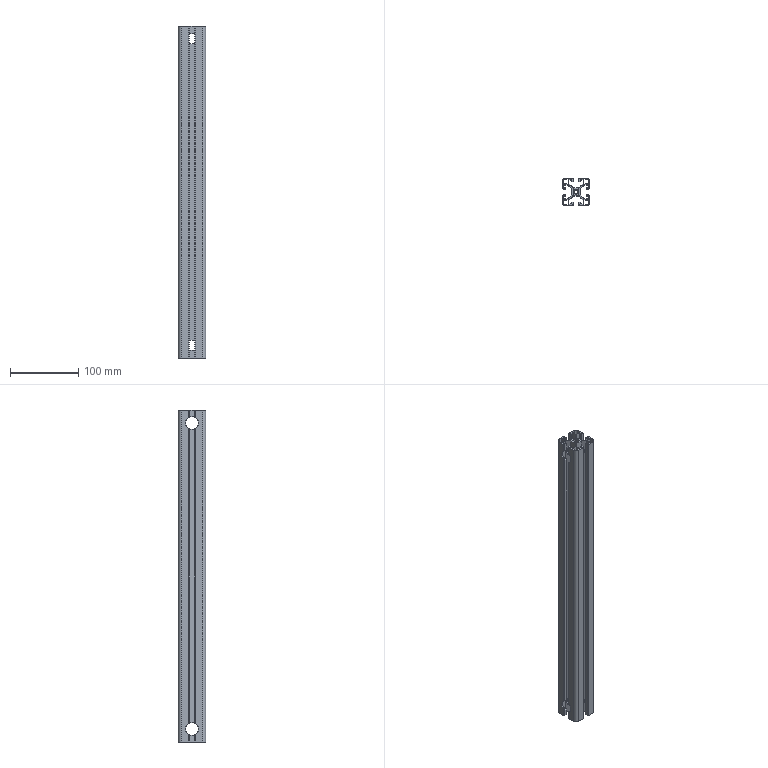Part | SolidWorks | features BaseBody 1, HoleWzd 1, MoveFace 1 | 1 solid | 235 faces | box 40 x 40 x 488 mm | volume 205502 mm3 | plane 166 | cylinder 69 | commonest cylinder face diameters 1.5 x18 2 x16 6.8 x15 19 x12 6.6 x4 9 x4